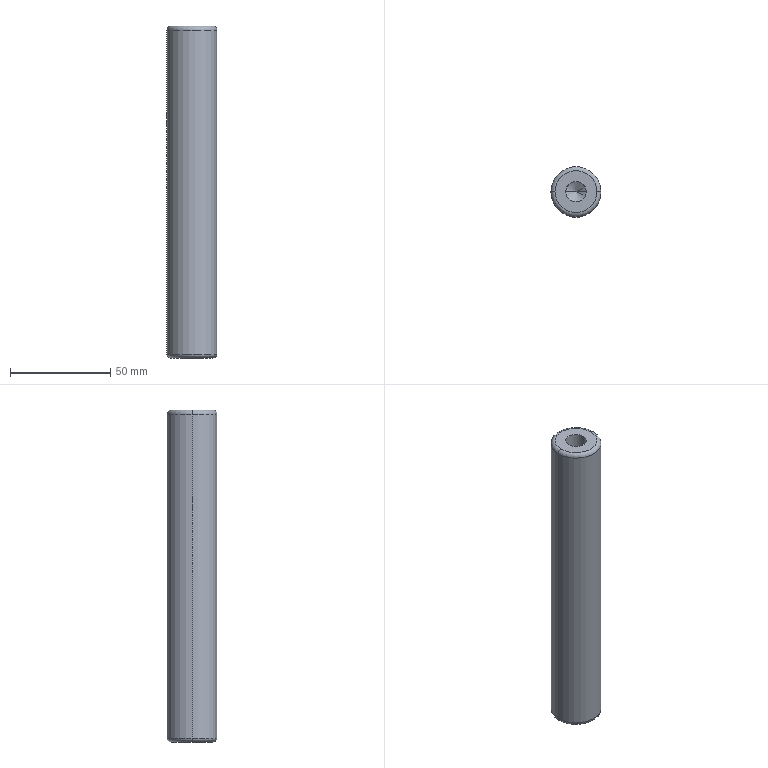Part | SolidWorks | features HoleWzd 2, Extrusion 1, Fillet 1 | 1 solid | 16 faces | box 25 x 25 x 166 mm | volume 76285 mm3 | cylinder 6 | cone 4 | torus 4 | plane 2 | commonest cylinder face diameters 10.2 x4 25 x2
STEP:
#1=CARTESIAN_POINT('',(5.1,0.,30.));
#2=VERTEX_POINT('',#1);
#3=CARTESIAN_POINT('',(-5.1,0.,30.));
#4=VERTEX_POINT('',#3);
#5=CARTESIAN_POINT('',(0.,0.,30.));
#6=DIRECTION('',(0.,0.,-1.));
#7=DIRECTION('',(-1.,0.,0.));
#8=AXIS2_PLACEMENT_3D('',#5,#6,#7);
#9=CIRCLE('',#8,5.1);
#10=EDGE_CURVE('',#2,#4,#9,.T.);
#11=ORIENTED_EDGE('',*,*,#10,.F.);
#12=CARTESIAN_POINT('',(5.1,0.,0.));
#13=VERTEX_POINT('',#12);
#14=CARTESIAN_POINT('',(5.1,0.,0.));
#15=DIRECTION('',(0.,0.,-1.));
#16=VECTOR('',#15,1000.);
#17=LINE('',#14,#16);
#18=EDGE_CURVE('',#2,#13,#17,.T.);
#19=ORIENTED_EDGE('',*,*,#18,.T.);
#20=CARTESIAN_POINT('',(-5.1,0.,0.));
#21=VERTEX_POINT('',#20);
#22=CARTESIAN_POINT('',(0.,0.,0.));
#23=DIRECTION('',(0.,0.,-1.));
#24=DIRECTION('',(-1.,0.,0.));
#25=AXIS2_PLACEMENT_3D('',#22,#23,#24);
#26=CIRCLE('',#25,5.1);
#27=EDGE_CURVE('',#13,#21,#26,.T.);
#28=ORIENTED_EDGE('',*,*,#27,.T.);
#29=CARTESIAN_POINT('',(-5.1,0.,0.));
#30=DIRECTION('',(0.,0.,-1.));
#31=VECTOR('',#30,1000.);
#32=LINE('',#29,#31);
#33=EDGE_CURVE('',#4,#21,#32,.T.);
#34=ORIENTED_EDGE('',*,*,#33,.F.);
#35=EDGE_LOOP('',(#11,#19,#28,#34));
#36=FACE_OUTER_BOUND('',#35,.T.);
#37=CARTESIAN_POINT('',(0.,0.,0.));
#38=DIRECTION('',(0.,0.,-1.));
#39=DIRECTION('',(-1.,0.,0.));
#40=AXIS2_PLACEMENT_3D('',#37,#38,#39);
#41=CYLINDRICAL_SURFACE('',#40,5.1);
#42=ADVANCED_FACE('',(#36),#41,.F.);
#43=CARTESIAN_POINT('',(0.,0.,33.064));
#44=VERTEX_POINT('',#43);
#45=CARTESIAN_POINT('',(-5.1,0.,30.));
#46=DIRECTION('',(-0.8572,0.,-0.515));
#47=VECTOR('',#46,1000.);
#48=LINE('',#45,#47);
#49=EDGE_CURVE('',#44,#4,#48,.T.);
#50=ORIENTED_EDGE('',*,*,#49,.F.);
#51=CARTESIAN_POINT('',(5.1,0.,30.));
#52=DIRECTION('',(0.8572,0.,-0.515));
#53=VECTOR('',#52,1000.);
#54=LINE('',#51,#53);
#55=EDGE_CURVE('',#44,#2,#54,.T.);
#56=ORIENTED_EDGE('',*,*,#55,.T.);
#57=ORIENTED_EDGE('',*,*,#10,.T.);
#58=EDGE_LOOP('',(#50,#56,#57));
#59=FACE_OUTER_BOUND('',#58,.T.);
#60=CARTESIAN_POINT('',(0.,0.,30.));
#61=DIRECTION('',(0.,0.,-1.));
#62=DIRECTION('',(-1.,0.,0.));
#63=AXIS2_PLACEMENT_3D('',#60,#61,#62);
#64=CONICAL_SURFACE('',#63,5.1,1.03);
#65=ADVANCED_FACE('',(#59),#64,.F.);
#66=CARTESIAN_POINT('',(-5.1,0.,136.));
#67=VERTEX_POINT('',#66);
#68=CARTESIAN_POINT('',(5.1,0.,136.));
#69=VERTEX_POINT('',#68);
#70=CARTESIAN_POINT('',(0.,0.,136.));
#71=DIRECTION('',(0.,0.,1.));
#72=DIRECTION('',(1.,0.,0.));
#73=AXIS2_PLACEMENT_3D('',#70,#71,#72);
#74=CIRCLE('',#73,5.1);
#75=EDGE_CURVE('',#67,#69,#74,.T.);
#76=ORIENTED_EDGE('',*,*,#75,.F.);
#77=CARTESIAN_POINT('',(-5.1,0.,166.));
#78=VERTEX_POINT('',#77);
#79=CARTESIAN_POINT('',(-5.1,0.,166.));
#80=DIRECTION('',(0.,0.,1.));
#81=VECTOR('',#80,1000.);
#82=LINE('',#79,#81);
#83=EDGE_CURVE('',#67,#78,#82,.T.);
#84=ORIENTED_EDGE('',*,*,#83,.T.);
#85=CARTESIAN_POINT('',(5.1,0.,166.));
#86=VERTEX_POINT('',#85);
#87=CARTESIAN_POINT('',(0.,0.,166.));
#88=DIRECTION('',(0.,0.,1.));
#89=DIRECTION('',(1.,0.,0.));
#90=AXIS2_PLACEMENT_3D('',#87,#88,#89);
#91=CIRCLE('',#90,5.1);
#92=EDGE_CURVE('',#78,#86,#91,.T.);
#93=ORIENTED_EDGE('',*,*,#92,.T.);
#94=CARTESIAN_POINT('',(5.1,0.,166.));
#95=DIRECTION('',(0.,0.,1.));
#96=VECTOR('',#95,1000.);
#97=LINE('',#94,#96);
#98=EDGE_CURVE('',#69,#86,#97,.T.);
#99=ORIENTED_EDGE('',*,*,#98,.F.);
#100=EDGE_LOOP('',(#76,#84,#93,#99));
#101=FACE_OUTER_BOUND('',#100,.T.);
#102=CARTESIAN_POINT('',(0.,0.,166.));
#103=DIRECTION('',(0.,0.,1.));
#104=DIRECTION('',(1.,0.,0.));
#105=AXIS2_PLACEMENT_3D('',#102,#103,#104);
#106=CYLINDRICAL_SURFACE('',#105,5.1);
#107=ADVANCED_FACE('',(#101),#106,.F.);
#108=CARTESIAN_POINT('',(0.,0.,132.936));
#109=VERTEX_POINT('',#108);
#110=CARTESIAN_POINT('',(5.1,0.,136.));
#111=DIRECTION('',(0.8572,0.,0.515));
#112=VECTOR('',#111,1000.);
#113=LINE('',#110,#112);
#114=EDGE_CURVE('',#109,#69,#113,.T.);
#115=ORIENTED_EDGE('',*,*,#114,.F.);
#116=CARTESIAN_POINT('',(-5.1,0.,136.));
#117=DIRECTION('',(-0.8572,0.,0.515));
#118=VECTOR('',#117,1000.);
#119=LINE('',#116,#118);
#120=EDGE_CURVE('',#109,#67,#119,.T.);
#121=ORIENTED_EDGE('',*,*,#120,.T.);
#122=ORIENTED_EDGE('',*,*,#75,.T.);
#123=EDGE_LOOP('',(#115,#121,#122));
#124=FACE_OUTER_BOUND('',#123,.T.);
#125=CARTESIAN_POINT('',(0.,0.,136.));
#126=DIRECTION('',(0.,0.,1.));
#127=DIRECTION('',(1.,0.,0.));
#128=AXIS2_PLACEMENT_3D('',#125,#126,#127);
#129=CONICAL_SURFACE('',#128,5.1,1.03);
#130=ADVANCED_FACE('',(#124),#129,.F.);
#131=CARTESIAN_POINT('',(-12.5,0.,164.));
#132=VERTEX_POINT('',#131);
#133=CARTESIAN_POINT('',(12.5,0.,164.));
#134=VERTEX_POINT('',#133);
#135=CARTESIAN_POINT('',(0.,0.,164.));
#136=DIRECTION('',(0.,0.,-1.));
#137=DIRECTION('',(1.,0.,0.));
#138=AXIS2_PLACEMENT_3D('',#135,#136,#137);
#139=CIRCLE('',#138,12.5);
#140=EDGE_CURVE('',#132,#134,#139,.T.);
#141=ORIENTED_EDGE('',*,*,#140,.F.);
#142=CARTESIAN_POINT('',(-10.5,0.,166.));
#143=VERTEX_POINT('',#142);
#144=CARTESIAN_POINT('',(-10.5,0.,164.));
#145=DIRECTION('',(0.,1.,0.));
#146=DIRECTION('',(-1.,0.,0.));
#147=AXIS2_PLACEMENT_3D('',#144,#145,#146);
#148=CIRCLE('',#147,2.);
#149=EDGE_CURVE('',#132,#143,#148,.T.);
#150=ORIENTED_EDGE('',*,*,#149,.T.);
#151=CARTESIAN_POINT('',(10.5,0.,166.));
#152=VERTEX_POINT('',#151);
#153=CARTESIAN_POINT('',(0.,0.,166.));
#154=DIRECTION('',(0.,0.,1.));
#155=DIRECTION('',(1.,0.,0.));
#156=AXIS2_PLACEMENT_3D('',#153,#154,#155);
#157=CIRCLE('',#156,10.5);
#158=EDGE_CURVE('',#152,#143,#157,.T.);
#159=ORIENTED_EDGE('',*,*,#158,.F.);
#160=CARTESIAN_POINT('',(10.5,0.,164.));
#161=DIRECTION('',(0.,-1.,0.));
#162=DIRECTION('',(0.,0.,-1.));
#163=AXIS2_PLACEMENT_3D('',#160,#161,#162);
#164=CIRCLE('',#163,2.);
#165=EDGE_CURVE('',#134,#152,#164,.T.);
#166=ORIENTED_EDGE('',*,*,#165,.F.);
#167=EDGE_LOOP('',(#141,#150,#159,#166));
#168=FACE_OUTER_BOUND('',#167,.T.);
#169=CARTESIAN_POINT('',(0.,0.,164.));
#170=DIRECTION('',(0.,0.,1.));
#171=DIRECTION('',(1.,0.,0.));
#172=AXIS2_PLACEMENT_3D('',#169,#170,#171);
#173=TOROIDAL_SURFACE('',#172,10.5,2.);
#174=ADVANCED_FACE('',(#168),#173,.T.);
#175=CARTESIAN_POINT('',(-10.5,0.,0.));
#176=VERTEX_POINT('',#175);
#177=CARTESIAN_POINT('',(10.5,0.,0.));
#178=VERTEX_POINT('',#177);
#179=CARTESIAN_POINT('',(0.,0.,0.));
#180=DIRECTION('',(0.,0.,-1.));
#181=DIRECTION('',(1.,0.,0.));
#182=AXIS2_PLACEMENT_3D('',#179,#180,#181);
#183=CIRCLE('',#182,10.5);
#184=EDGE_CURVE('',#176,#178,#183,.T.);
#185=ORIENTED_EDGE('',*,*,#184,.F.);
#186=CARTESIAN_POINT('',(-12.5,0.,2.));
#187=VERTEX_POINT('',#186);
#188=CARTESIAN_POINT('',(-10.5,0.,2.));
#189=DIRECTION('',(0.,1.,0.));
#190=DIRECTION('',(-1.,0.,0.));
#191=AXIS2_PLACEMENT_3D('',#188,#189,#190);
#192=CIRCLE('',#191,2.);
#193=EDGE_CURVE('',#176,#187,#192,.T.);
#194=ORIENTED_EDGE('',*,*,#193,.T.);
#195=CARTESIAN_POINT('',(12.5,0.,2.));
#196=VERTEX_POINT('',#195);
#197=CARTESIAN_POINT('',(0.,0.,2.));
#198=DIRECTION('',(0.,0.,1.));
#199=DIRECTION('',(1.,0.,0.));
#200=AXIS2_PLACEMENT_3D('',#197,#198,#199);
#201=CIRCLE('',#200,12.5);
#202=EDGE_CURVE('',#196,#187,#201,.T.);
#203=ORIENTED_EDGE('',*,*,#202,.F.);
#204=CARTESIAN_POINT('',(10.5,0.,2.));
#205=DIRECTION('',(0.,-1.,0.));
#206=DIRECTION('',(0.,0.,-1.));
#207=AXIS2_PLACEMENT_3D('',#204,#205,#206);
#208=CIRCLE('',#207,2.);
#209=EDGE_CURVE('',#178,#196,#208,.T.);
#210=ORIENTED_EDGE('',*,*,#209,.F.);
#211=EDGE_LOOP('',(#185,#194,#203,#210));
#212=FACE_OUTER_BOUND('',#211,.T.);
#213=CARTESIAN_POINT('',(0.,0.,2.));
#214=DIRECTION('',(0.,0.,1.));
#215=DIRECTION('',(1.,0.,0.));
#216=AXIS2_PLACEMENT_3D('',#213,#214,#215);
#217=TOROIDAL_SURFACE('',#216,10.5,2.);
#218=ADVANCED_FACE('',(#212),#217,.T.);
#219=ORIENTED_EDGE('',*,*,#140,.T.);
#220=CARTESIAN_POINT('',(12.5,0.,166.));
#221=DIRECTION('',(0.,0.,-1.));
#222=VECTOR('',#221,1000.);
#223=LINE('',#220,#222);
#224=EDGE_CURVE('',#134,#196,#223,.T.);
#225=ORIENTED_EDGE('',*,*,#224,.T.);
#226=ORIENTED_EDGE('',*,*,#202,.T.);
#227=CARTESIAN_POINT('',(-12.5,0.,166.));
#228=DIRECTION('',(0.,0.,-1.));
#229=VECTOR('',#228,1000.);
#230=LINE('',#227,#229);
#231=EDGE_CURVE('',#132,#187,#230,.T.);
#232=ORIENTED_EDGE('',*,*,#231,.F.);
#233=EDGE_LOOP('',(#219,#225,#226,#232));
#234=FACE_OUTER_BOUND('',#233,.T.);
#235=CARTESIAN_POINT('',(0.,0.,166.));
#236=DIRECTION('',(0.,0.,-1.));
#237=DIRECTION('',(-1.,0.,0.));
#238=AXIS2_PLACEMENT_3D('',#235,#236,#237);
#239=CYLINDRICAL_SURFACE('',#238,12.5);
#240=ADVANCED_FACE('',(#234),#239,.T.);
#241=ORIENTED_EDGE('',*,*,#224,.F.);
#242=CARTESIAN_POINT('',(0.,0.,164.));
#243=DIRECTION('',(0.,0.,-1.));
#244=DIRECTION('',(1.,0.,0.));
#245=AXIS2_PLACEMENT_3D('',#242,#243,#244);
#246=CIRCLE('',#245,12.5);
#247=EDGE_CURVE('',#134,#132,#246,.T.);
#248=ORIENTED_EDGE('',*,*,#247,.T.);
#249=ORIENTED_EDGE('',*,*,#231,.T.);
#250=CARTESIAN_POINT('',(0.,0.,2.));
#251=DIRECTION('',(0.,0.,1.));
#252=DIRECTION('',(1.,0.,0.));
#253=AXIS2_PLACEMENT_3D('',#250,#251,#252);
#254=CIRCLE('',#253,12.5);
#255=EDGE_CURVE('',#187,#196,#254,.T.);
#256=ORIENTED_EDGE('',*,*,#255,.T.);
#257=EDGE_LOOP('',(#241,#248,#249,#256));
#258=FACE_OUTER_BOUND('',#257,.T.);
#259=CARTESIAN_POINT('',(0.,0.,166.));
#260=DIRECTION('',(0.,0.,-1.));
#261=DIRECTION('',(-1.,0.,0.));
#262=AXIS2_PLACEMENT_3D('',#259,#260,#261);
#263=CYLINDRICAL_SURFACE('',#262,12.5);
#264=ADVANCED_FACE('',(#258),#263,.T.);
#265=CARTESIAN_POINT('',(0.,0.,166.));
#266=DIRECTION('',(0.,0.,1.));
#267=DIRECTION('',(1.,0.,0.));
#268=AXIS2_PLACEMENT_3D('',#265,#266,#267);
#269=CIRCLE('',#268,5.1);
#270=EDGE_CURVE('',#86,#78,#269,.T.);
#271=ORIENTED_EDGE('',*,*,#270,.F.);
#272=ORIENTED_EDGE('',*,*,#92,.F.);
#273=EDGE_LOOP('',(#271,#272));
#274=FACE_BOUND('',#273,.T.);
#275=ORIENTED_EDGE('',*,*,#158,.T.);
#276=CARTESIAN_POINT('',(0.,0.,166.));
#277=DIRECTION('',(0.,0.,1.));
#278=DIRECTION('',(1.,0.,0.));
#279=AXIS2_PLACEMENT_3D('',#276,#277,#278);
#280=CIRCLE('',#279,10.5);
#281=EDGE_CURVE('',#143,#152,#280,.T.);
#282=ORIENTED_EDGE('',*,*,#281,.T.);
#283=EDGE_LOOP('',(#275,#282));
#284=FACE_OUTER_BOUND('',#283,.T.);
#285=CARTESIAN_POINT('',(0.,0.,166.));
#286=DIRECTION('',(0.,0.,1.));
#287=DIRECTION('',(1.,0.,0.));
#288=AXIS2_PLACEMENT_3D('',#285,#286,#287);
#289=PLANE('',#288);
#290=ADVANCED_FACE('',(#274,#284),#289,.T.);
#291=CARTESIAN_POINT('',(0.,0.,0.));
#292=DIRECTION('',(0.,0.,-1.));
#293=DIRECTION('',(-1.,0.,0.));
#294=AXIS2_PLACEMENT_3D('',#291,#292,#293);
#295=CIRCLE('',#294,5.1);
#296=EDGE_CURVE('',#21,#13,#295,.T.);
#297=ORIENTED_EDGE('',*,*,#296,.F.);
#298=ORIENTED_EDGE('',*,*,#27,.F.);
#299=EDGE_LOOP('',(#297,#298));
#300=FACE_BOUND('',#299,.T.);
#301=CARTESIAN_POINT('',(0.,0.,0.));
#302=DIRECTION('',(0.,0.,-1.));
#303=DIRECTION('',(1.,0.,0.));
#304=AXIS2_PLACEMENT_3D('',#301,#302,#303);
#305=CIRCLE('',#304,10.5);
#306=EDGE_CURVE('',#178,#176,#305,.T.);
#307=ORIENTED_EDGE('',*,*,#306,.T.);
#308=ORIENTED_EDGE('',*,*,#184,.T.);
#309=EDGE_LOOP('',(#307,#308));
#310=FACE_OUTER_BOUND('',#309,.T.);
#311=CARTESIAN_POINT('',(0.,0.,0.));
#312=DIRECTION('',(0.,0.,1.));
#313=DIRECTION('',(1.,0.,0.));
#314=AXIS2_PLACEMENT_3D('',#311,#312,#313);
#315=PLANE('',#314);
#316=ADVANCED_FACE('',(#300,#310),#315,.F.);
#317=ORIENTED_EDGE('',*,*,#193,.F.);
#318=ORIENTED_EDGE('',*,*,#306,.F.);
#319=ORIENTED_EDGE('',*,*,#209,.T.);
#320=ORIENTED_EDGE('',*,*,#255,.F.);
#321=EDGE_LOOP('',(#317,#318,#319,#320));
#322=FACE_OUTER_BOUND('',#321,.T.);
#323=CARTESIAN_POINT('',(0.,0.,2.));
#324=DIRECTION('',(0.,0.,1.));
#325=DIRECTION('',(1.,0.,0.));
#326=AXIS2_PLACEMENT_3D('',#323,#324,#325);
#327=TOROIDAL_SURFACE('',#326,10.5,2.);
#328=ADVANCED_FACE('',(#322),#327,.T.);
#329=ORIENTED_EDGE('',*,*,#149,.F.);
#330=ORIENTED_EDGE('',*,*,#247,.F.);
#331=ORIENTED_EDGE('',*,*,#165,.T.);
#332=ORIENTED_EDGE('',*,*,#281,.F.);
#333=EDGE_LOOP('',(#329,#330,#331,#332));
#334=FACE_OUTER_BOUND('',#333,.T.);
#335=CARTESIAN_POINT('',(0.,0.,164.));
#336=DIRECTION('',(0.,0.,1.));
#337=DIRECTION('',(1.,0.,0.));
#338=AXIS2_PLACEMENT_3D('',#335,#336,#337);
#339=TOROIDAL_SURFACE('',#338,10.5,2.);
#340=ADVANCED_FACE('',(#334),#339,.T.);
#341=ORIENTED_EDGE('',*,*,#120,.F.);
#342=ORIENTED_EDGE('',*,*,#114,.T.);
#343=CARTESIAN_POINT('',(0.,0.,136.));
#344=DIRECTION('',(0.,0.,1.));
#345=DIRECTION('',(1.,0.,0.));
#346=AXIS2_PLACEMENT_3D('',#343,#344,#345);
#347=CIRCLE('',#346,5.1);
#348=EDGE_CURVE('',#69,#67,#347,.T.);
#349=ORIENTED_EDGE('',*,*,#348,.T.);
#350=EDGE_LOOP('',(#341,#342,#349));
#351=FACE_OUTER_BOUND('',#350,.T.);
#352=CARTESIAN_POINT('',(0.,0.,136.));
#353=DIRECTION('',(0.,0.,1.));
#354=DIRECTION('',(1.,0.,0.));
#355=AXIS2_PLACEMENT_3D('',#352,#353,#354);
#356=CONICAL_SURFACE('',#355,5.1,1.03);
#357=ADVANCED_FACE('',(#351),#356,.F.);
#358=ORIENTED_EDGE('',*,*,#83,.F.);
#359=ORIENTED_EDGE('',*,*,#348,.F.);
#360=ORIENTED_EDGE('',*,*,#98,.T.);
#361=ORIENTED_EDGE('',*,*,#270,.T.);
#362=EDGE_LOOP('',(#358,#359,#360,#361));
#363=FACE_OUTER_BOUND('',#362,.T.);
#364=CARTESIAN_POINT('',(0.,0.,166.));
#365=DIRECTION('',(0.,0.,1.));
#366=DIRECTION('',(1.,0.,0.));
#367=AXIS2_PLACEMENT_3D('',#364,#365,#366);
#368=CYLINDRICAL_SURFACE('',#367,5.1);
#369=ADVANCED_FACE('',(#363),#368,.F.);
#370=ORIENTED_EDGE('',*,*,#55,.F.);
#371=ORIENTED_EDGE('',*,*,#49,.T.);
#372=CARTESIAN_POINT('',(0.,0.,30.));
#373=DIRECTION('',(0.,0.,-1.));
#374=DIRECTION('',(-1.,0.,0.));
#375=AXIS2_PLACEMENT_3D('',#372,#373,#374);
#376=CIRCLE('',#375,5.1);
#377=EDGE_CURVE('',#4,#2,#376,.T.);
#378=ORIENTED_EDGE('',*,*,#377,.T.);
#379=EDGE_LOOP('',(#370,#371,#378));
#380=FACE_OUTER_BOUND('',#379,.T.);
#381=CARTESIAN_POINT('',(0.,0.,30.));
#382=DIRECTION('',(0.,0.,-1.));
#383=DIRECTION('',(-1.,0.,0.));
#384=AXIS2_PLACEMENT_3D('',#381,#382,#383);
#385=CONICAL_SURFACE('',#384,5.1,1.03);
#386=ADVANCED_FACE('',(#380),#385,.F.);
#387=ORIENTED_EDGE('',*,*,#18,.F.);
#388=ORIENTED_EDGE('',*,*,#377,.F.);
#389=ORIENTED_EDGE('',*,*,#33,.T.);
#390=ORIENTED_EDGE('',*,*,#296,.T.);
#391=EDGE_LOOP('',(#387,#388,#389,#390));
#392=FACE_OUTER_BOUND('',#391,.T.);
#393=CARTESIAN_POINT('',(0.,0.,0.));
#394=DIRECTION('',(0.,0.,-1.));
#395=DIRECTION('',(-1.,0.,0.));
#396=AXIS2_PLACEMENT_3D('',#393,#394,#395);
#397=CYLINDRICAL_SURFACE('',#396,5.1);
#398=ADVANCED_FACE('',(#392),#397,.F.);
#399=CLOSED_SHELL('',(#42,#65,#107,#130,#174,#218,#240,#264,#290,#316,#328,#340,#357,#369,#386,#398));
#400=MANIFOLD_SOLID_BREP('',#399);
#401=CARTESIAN_POINT('',(0.,0.,0.));
#402=DIRECTION('',(0.,0.,1.));
#403=DIRECTION('',(1.,0.,0.));
#404=AXIS2_PLACEMENT_3D('',#401,#402,#403);
#405=(LENGTH_UNIT()NAMED_UNIT(*)SI_UNIT(.MILLI.,.METRE.));
#406=UNCERTAINTY_MEASURE_WITH_UNIT(LENGTH_MEASURE(0.00001),#405,'','');
#407=(NAMED_UNIT(*)PLANE_ANGLE_UNIT()SI_UNIT($,.RADIAN.));
#408=(NAMED_UNIT(*)SI_UNIT($,.STERADIAN.)SOLID_ANGLE_UNIT());
#409=(GEOMETRIC_REPRESENTATION_CONTEXT(3)GLOBAL_UNCERTAINTY_ASSIGNED_CONTEXT((#406))GLOBAL_UNIT_ASSIGNED_CONTEXT((#405,#407,#408))REPRESENTATION_CONTEXT('',''));
#410=ADVANCED_BREP_SHAPE_REPRESENTATION('',(#400,#404),#409);